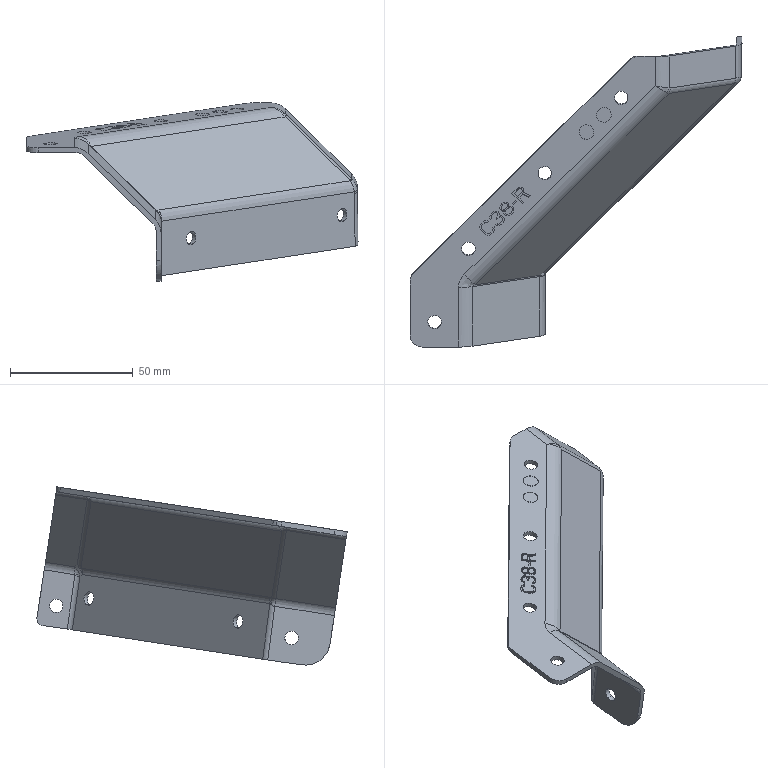Part | SolidWorks | features BaseBody 1 | 1 solid | 294 faces | box 135.25 x 126.407 x 72.597 mm | volume 24693 mm3 | plane 226 | cylinder 50 | spline 18 | commonest cylinder face diameters 5.5 x16 6 x9 16 x9 9 x7 10 x4 2 x2